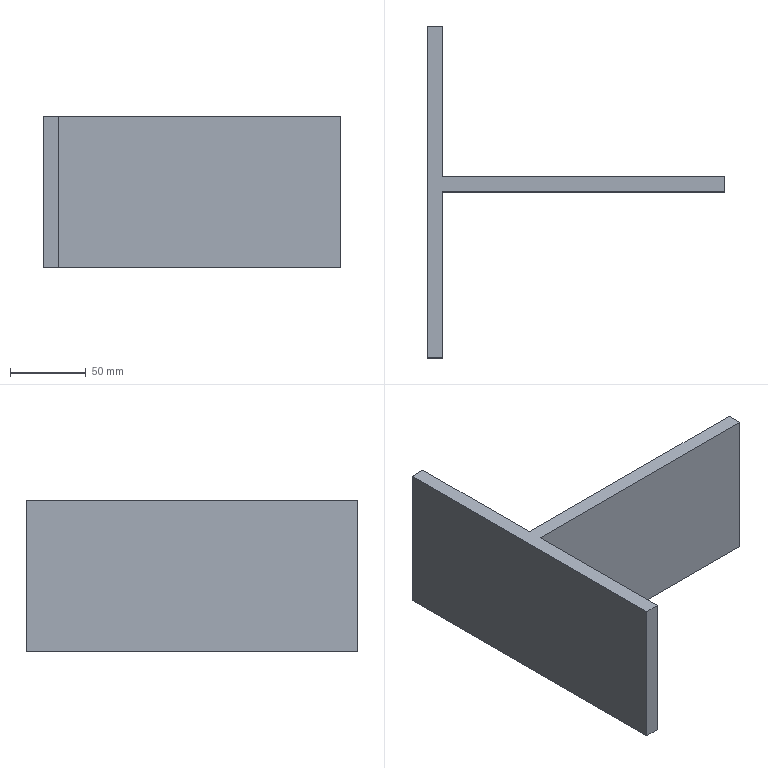Part | STEP file | Mirror slide plate 3 | 1 solid | 10 faces | box 196 x 218.322 x 100 mm | volume 404322 mm3 | plane 10
STEP:
#1=CARTESIAN_POINT('',(93.,0.,-50.));
#2=VERTEX_POINT('',#1);
#3=CARTESIAN_POINT('',(93.,0.,50.));
#4=VERTEX_POINT('',#3);
#5=CARTESIAN_POINT('',(93.,0.,50.));
#6=DIRECTION('',(0.,0.,1.));
#7=VECTOR('',#6,1000.);
#8=LINE('',#5,#7);
#9=EDGE_CURVE('',#2,#4,#8,.T.);
#10=ORIENTED_EDGE('',*,*,#9,.F.);
#11=CARTESIAN_POINT('',(93.,10.,-50.));
#12=VERTEX_POINT('',#11);
#13=CARTESIAN_POINT('',(93.,10.,-50.));
#14=DIRECTION('',(0.,-1.,0.));
#15=VECTOR('',#14,1000.);
#16=LINE('',#13,#15);
#17=EDGE_CURVE('',#12,#2,#16,.T.);
#18=ORIENTED_EDGE('',*,*,#17,.F.);
#19=CARTESIAN_POINT('',(93.,10.,50.));
#20=VERTEX_POINT('',#19);
#21=CARTESIAN_POINT('',(93.,10.,50.));
#22=DIRECTION('',(0.,0.,1.));
#23=VECTOR('',#22,1000.);
#24=LINE('',#21,#23);
#25=EDGE_CURVE('',#12,#20,#24,.T.);
#26=ORIENTED_EDGE('',*,*,#25,.T.);
#27=CARTESIAN_POINT('',(93.,10.,50.));
#28=DIRECTION('',(0.,-1.,0.));
#29=VECTOR('',#28,1000.);
#30=LINE('',#27,#29);
#31=EDGE_CURVE('',#20,#4,#30,.T.);
#32=ORIENTED_EDGE('',*,*,#31,.T.);
#33=EDGE_LOOP('',(#10,#18,#26,#32));
#34=FACE_OUTER_BOUND('',#33,.T.);
#35=CARTESIAN_POINT('',(93.,10.,50.));
#36=DIRECTION('',(-1.,0.,0.));
#37=DIRECTION('',(0.,0.,-1.));
#38=AXIS2_PLACEMENT_3D('',#35,#36,#37);
#39=PLANE('',#38);
#40=ADVANCED_FACE('',(#34),#39,.F.);
#41=CARTESIAN_POINT('',(-93.,0.,50.));
#42=VERTEX_POINT('',#41);
#43=CARTESIAN_POINT('',(-93.,0.,50.));
#44=DIRECTION('',(-1.,0.,0.));
#45=VECTOR('',#44,1000.);
#46=LINE('',#43,#45);
#47=EDGE_CURVE('',#4,#42,#46,.T.);
#48=ORIENTED_EDGE('',*,*,#47,.F.);
#49=ORIENTED_EDGE('',*,*,#31,.F.);
#50=CARTESIAN_POINT('',(-93.,10.,50.));
#51=VERTEX_POINT('',#50);
#52=CARTESIAN_POINT('',(-93.,10.,50.));
#53=DIRECTION('',(-1.,0.,0.));
#54=VECTOR('',#53,1000.);
#55=LINE('',#52,#54);
#56=EDGE_CURVE('',#20,#51,#55,.T.);
#57=ORIENTED_EDGE('',*,*,#56,.T.);
#58=CARTESIAN_POINT('',(-93.,109.161,50.));
#59=VERTEX_POINT('',#58);
#60=CARTESIAN_POINT('',(-93.,109.161,50.));
#61=DIRECTION('',(0.,-1.,0.));
#62=VECTOR('',#61,1000.);
#63=LINE('',#60,#62);
#64=EDGE_CURVE('',#59,#51,#63,.T.);
#65=ORIENTED_EDGE('',*,*,#64,.F.);
#66=CARTESIAN_POINT('',(-103.,109.161,50.));
#67=VERTEX_POINT('',#66);
#68=CARTESIAN_POINT('',(-103.,109.161,50.));
#69=DIRECTION('',(1.,0.,0.));
#70=VECTOR('',#69,1000.);
#71=LINE('',#68,#70);
#72=EDGE_CURVE('',#67,#59,#71,.T.);
#73=ORIENTED_EDGE('',*,*,#72,.F.);
#74=CARTESIAN_POINT('',(-103.,-109.161,50.));
#75=VERTEX_POINT('',#74);
#76=CARTESIAN_POINT('',(-103.,109.161,50.));
#77=DIRECTION('',(0.,-1.,0.));
#78=VECTOR('',#77,1000.);
#79=LINE('',#76,#78);
#80=EDGE_CURVE('',#67,#75,#79,.T.);
#81=ORIENTED_EDGE('',*,*,#80,.T.);
#82=CARTESIAN_POINT('',(-93.,-109.161,50.));
#83=VERTEX_POINT('',#82);
#84=CARTESIAN_POINT('',(-103.,-109.161,50.));
#85=DIRECTION('',(1.,0.,0.));
#86=VECTOR('',#85,1000.);
#87=LINE('',#84,#86);
#88=EDGE_CURVE('',#75,#83,#87,.T.);
#89=ORIENTED_EDGE('',*,*,#88,.T.);
#90=CARTESIAN_POINT('',(-93.,109.161,50.));
#91=DIRECTION('',(0.,-1.,0.));
#92=VECTOR('',#91,1000.);
#93=LINE('',#90,#92);
#94=EDGE_CURVE('',#42,#83,#93,.T.);
#95=ORIENTED_EDGE('',*,*,#94,.F.);
#96=EDGE_LOOP('',(#48,#49,#57,#65,#73,#81,#89,#95));
#97=FACE_OUTER_BOUND('',#96,.T.);
#98=CARTESIAN_POINT('',(-93.,10.,50.));
#99=DIRECTION('',(0.,0.,-1.));
#100=DIRECTION('',(1.,0.,0.));
#101=AXIS2_PLACEMENT_3D('',#98,#99,#100);
#102=PLANE('',#101);
#103=ADVANCED_FACE('',(#97),#102,.F.);
#104=CARTESIAN_POINT('',(-93.,0.,-50.));
#105=VERTEX_POINT('',#104);
#106=CARTESIAN_POINT('',(-93.,0.,-50.));
#107=DIRECTION('',(1.,0.,0.));
#108=VECTOR('',#107,1000.);
#109=LINE('',#106,#108);
#110=EDGE_CURVE('',#105,#2,#109,.T.);
#111=ORIENTED_EDGE('',*,*,#110,.F.);
#112=CARTESIAN_POINT('',(-93.,-109.161,-50.));
#113=VERTEX_POINT('',#112);
#114=CARTESIAN_POINT('',(-93.,109.161,-50.));
#115=DIRECTION('',(0.,1.,0.));
#116=VECTOR('',#115,1000.);
#117=LINE('',#114,#116);
#118=EDGE_CURVE('',#113,#105,#117,.T.);
#119=ORIENTED_EDGE('',*,*,#118,.F.);
#120=CARTESIAN_POINT('',(-103.,-109.161,-50.));
#121=VERTEX_POINT('',#120);
#122=CARTESIAN_POINT('',(-103.,-109.161,-50.));
#123=DIRECTION('',(1.,0.,0.));
#124=VECTOR('',#123,1000.);
#125=LINE('',#122,#124);
#126=EDGE_CURVE('',#121,#113,#125,.T.);
#127=ORIENTED_EDGE('',*,*,#126,.F.);
#128=CARTESIAN_POINT('',(-103.,109.161,-50.));
#129=VERTEX_POINT('',#128);
#130=CARTESIAN_POINT('',(-103.,109.161,-50.));
#131=DIRECTION('',(0.,1.,0.));
#132=VECTOR('',#131,1000.);
#133=LINE('',#130,#132);
#134=EDGE_CURVE('',#121,#129,#133,.T.);
#135=ORIENTED_EDGE('',*,*,#134,.T.);
#136=CARTESIAN_POINT('',(-93.,109.161,-50.));
#137=VERTEX_POINT('',#136);
#138=CARTESIAN_POINT('',(-103.,109.161,-50.));
#139=DIRECTION('',(1.,0.,0.));
#140=VECTOR('',#139,1000.);
#141=LINE('',#138,#140);
#142=EDGE_CURVE('',#129,#137,#141,.T.);
#143=ORIENTED_EDGE('',*,*,#142,.T.);
#144=CARTESIAN_POINT('',(-93.,10.,-50.));
#145=VERTEX_POINT('',#144);
#146=CARTESIAN_POINT('',(-93.,109.161,-50.));
#147=DIRECTION('',(0.,1.,0.));
#148=VECTOR('',#147,1000.);
#149=LINE('',#146,#148);
#150=EDGE_CURVE('',#145,#137,#149,.T.);
#151=ORIENTED_EDGE('',*,*,#150,.F.);
#152=CARTESIAN_POINT('',(-93.,10.,-50.));
#153=DIRECTION('',(1.,0.,0.));
#154=VECTOR('',#153,1000.);
#155=LINE('',#152,#154);
#156=EDGE_CURVE('',#145,#12,#155,.T.);
#157=ORIENTED_EDGE('',*,*,#156,.T.);
#158=ORIENTED_EDGE('',*,*,#17,.T.);
#159=EDGE_LOOP('',(#111,#119,#127,#135,#143,#151,#157,#158));
#160=FACE_OUTER_BOUND('',#159,.T.);
#161=CARTESIAN_POINT('',(-93.,10.,-50.));
#162=DIRECTION('',(0.,0.,1.));
#163=DIRECTION('',(-1.,0.,0.));
#164=AXIS2_PLACEMENT_3D('',#161,#162,#163);
#165=PLANE('',#164);
#166=ADVANCED_FACE('',(#160),#165,.F.);
#167=ORIENTED_EDGE('',*,*,#25,.F.);
#168=ORIENTED_EDGE('',*,*,#156,.F.);
#169=CARTESIAN_POINT('',(-93.,10.,50.));
#170=DIRECTION('',(0.,0.,-1.));
#171=VECTOR('',#170,1000.);
#172=LINE('',#169,#171);
#173=EDGE_CURVE('',#51,#145,#172,.T.);
#174=ORIENTED_EDGE('',*,*,#173,.F.);
#175=ORIENTED_EDGE('',*,*,#56,.F.);
#176=EDGE_LOOP('',(#167,#168,#174,#175));
#177=FACE_OUTER_BOUND('',#176,.T.);
#178=CARTESIAN_POINT('',(0.,10.,0.));
#179=DIRECTION('',(0.,1.,0.));
#180=DIRECTION('',(0.,0.,-1.));
#181=AXIS2_PLACEMENT_3D('',#178,#179,#180);
#182=PLANE('',#181);
#183=ADVANCED_FACE('',(#177),#182,.T.);
#184=ORIENTED_EDGE('',*,*,#9,.T.);
#185=ORIENTED_EDGE('',*,*,#47,.T.);
#186=CARTESIAN_POINT('',(-93.,0.,50.));
#187=DIRECTION('',(0.,0.,-1.));
#188=VECTOR('',#187,1000.);
#189=LINE('',#186,#188);
#190=EDGE_CURVE('',#42,#105,#189,.T.);
#191=ORIENTED_EDGE('',*,*,#190,.T.);
#192=ORIENTED_EDGE('',*,*,#110,.T.);
#193=EDGE_LOOP('',(#184,#185,#191,#192));
#194=FACE_OUTER_BOUND('',#193,.T.);
#195=CARTESIAN_POINT('',(0.,0.,0.));
#196=DIRECTION('',(0.,1.,0.));
#197=DIRECTION('',(0.,0.,-1.));
#198=AXIS2_PLACEMENT_3D('',#195,#196,#197);
#199=PLANE('',#198);
#200=ADVANCED_FACE('',(#194),#199,.F.);
#201=ORIENTED_EDGE('',*,*,#94,.T.);
#202=CARTESIAN_POINT('',(-93.,-109.161,50.));
#203=DIRECTION('',(0.,0.,-1.));
#204=VECTOR('',#203,1000.);
#205=LINE('',#202,#204);
#206=EDGE_CURVE('',#83,#113,#205,.T.);
#207=ORIENTED_EDGE('',*,*,#206,.T.);
#208=ORIENTED_EDGE('',*,*,#118,.T.);
#209=ORIENTED_EDGE('',*,*,#190,.F.);
#210=EDGE_LOOP('',(#201,#207,#208,#209));
#211=FACE_OUTER_BOUND('',#210,.T.);
#212=CARTESIAN_POINT('',(-93.,0.,0.));
#213=DIRECTION('',(-1.,0.,0.));
#214=DIRECTION('',(0.,0.,-1.));
#215=AXIS2_PLACEMENT_3D('',#212,#213,#214);
#216=PLANE('',#215);
#217=ADVANCED_FACE('',(#211),#216,.F.);
#218=CARTESIAN_POINT('',(-93.,109.161,50.));
#219=DIRECTION('',(0.,0.,1.));
#220=VECTOR('',#219,1000.);
#221=LINE('',#218,#220);
#222=EDGE_CURVE('',#137,#59,#221,.T.);
#223=ORIENTED_EDGE('',*,*,#222,.F.);
#224=ORIENTED_EDGE('',*,*,#142,.F.);
#225=CARTESIAN_POINT('',(-103.,109.161,50.));
#226=DIRECTION('',(0.,0.,1.));
#227=VECTOR('',#226,1000.);
#228=LINE('',#225,#227);
#229=EDGE_CURVE('',#129,#67,#228,.T.);
#230=ORIENTED_EDGE('',*,*,#229,.T.);
#231=ORIENTED_EDGE('',*,*,#72,.T.);
#232=EDGE_LOOP('',(#223,#224,#230,#231));
#233=FACE_OUTER_BOUND('',#232,.T.);
#234=CARTESIAN_POINT('',(-103.,109.161,50.));
#235=DIRECTION('',(0.,-1.,0.));
#236=DIRECTION('',(0.,0.,1.));
#237=AXIS2_PLACEMENT_3D('',#234,#235,#236);
#238=PLANE('',#237);
#239=ADVANCED_FACE('',(#233),#238,.F.);
#240=ORIENTED_EDGE('',*,*,#206,.F.);
#241=ORIENTED_EDGE('',*,*,#88,.F.);
#242=CARTESIAN_POINT('',(-103.,-109.161,50.));
#243=DIRECTION('',(0.,0.,-1.));
#244=VECTOR('',#243,1000.);
#245=LINE('',#242,#244);
#246=EDGE_CURVE('',#75,#121,#245,.T.);
#247=ORIENTED_EDGE('',*,*,#246,.T.);
#248=ORIENTED_EDGE('',*,*,#126,.T.);
#249=EDGE_LOOP('',(#240,#241,#247,#248));
#250=FACE_OUTER_BOUND('',#249,.T.);
#251=CARTESIAN_POINT('',(-103.,-109.161,50.));
#252=DIRECTION('',(0.,1.,0.));
#253=DIRECTION('',(0.,0.,-1.));
#254=AXIS2_PLACEMENT_3D('',#251,#252,#253);
#255=PLANE('',#254);
#256=ADVANCED_FACE('',(#250),#255,.F.);
#257=ORIENTED_EDGE('',*,*,#134,.F.);
#258=ORIENTED_EDGE('',*,*,#246,.F.);
#259=ORIENTED_EDGE('',*,*,#80,.F.);
#260=ORIENTED_EDGE('',*,*,#229,.F.);
#261=EDGE_LOOP('',(#257,#258,#259,#260));
#262=FACE_OUTER_BOUND('',#261,.T.);
#263=CARTESIAN_POINT('',(-103.,0.,0.));
#264=DIRECTION('',(-1.,0.,0.));
#265=DIRECTION('',(0.,0.,-1.));
#266=AXIS2_PLACEMENT_3D('',#263,#264,#265);
#267=PLANE('',#266);
#268=ADVANCED_FACE('',(#262),#267,.T.);
#269=ORIENTED_EDGE('',*,*,#173,.T.);
#270=ORIENTED_EDGE('',*,*,#150,.T.);
#271=ORIENTED_EDGE('',*,*,#222,.T.);
#272=ORIENTED_EDGE('',*,*,#64,.T.);
#273=EDGE_LOOP('',(#269,#270,#271,#272));
#274=FACE_OUTER_BOUND('',#273,.T.);
#275=CARTESIAN_POINT('',(-93.,0.,0.));
#276=DIRECTION('',(-1.,0.,0.));
#277=DIRECTION('',(0.,0.,-1.));
#278=AXIS2_PLACEMENT_3D('',#275,#276,#277);
#279=PLANE('',#278);
#280=ADVANCED_FACE('',(#274),#279,.F.);
#281=CLOSED_SHELL('',(#40,#103,#166,#183,#200,#217,#239,#256,#268,#280));
#282=MANIFOLD_SOLID_BREP('',#281);
#283=CARTESIAN_POINT('',(0.,0.,0.));
#284=DIRECTION('',(0.,0.,1.));
#285=DIRECTION('',(1.,0.,0.));
#286=AXIS2_PLACEMENT_3D('',#283,#284,#285);
#287=(LENGTH_UNIT()NAMED_UNIT(*)SI_UNIT(.MILLI.,.METRE.));
#288=UNCERTAINTY_MEASURE_WITH_UNIT(LENGTH_MEASURE(0.00001),#287,'','');
#289=(NAMED_UNIT(*)PLANE_ANGLE_UNIT()SI_UNIT($,.RADIAN.));
#290=(NAMED_UNIT(*)SI_UNIT($,.STERADIAN.)SOLID_ANGLE_UNIT());
#291=(GEOMETRIC_REPRESENTATION_CONTEXT(3)GLOBAL_UNCERTAINTY_ASSIGNED_CONTEXT((#288))GLOBAL_UNIT_ASSIGNED_CONTEXT((#287,#289,#290))REPRESENTATION_CONTEXT('',''));
#292=ADVANCED_BREP_SHAPE_REPRESENTATION('',(#282,#286),#291);